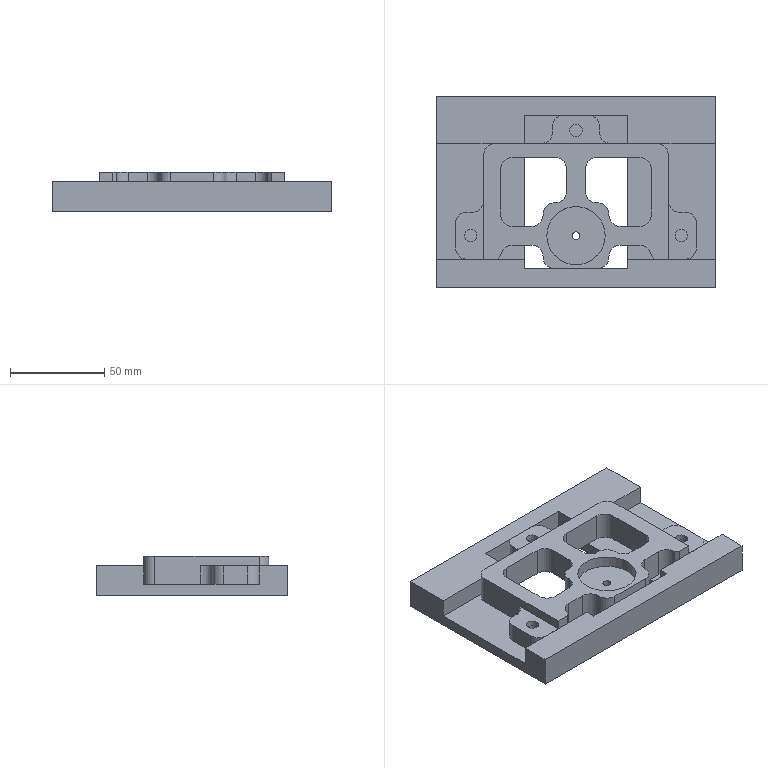NC program | NX | posted with a generic post | part box 148 x 101.5 x 21 mm
Lines 3456 to 5224 of 5700, first 1550 of 1759 lines:
(DRILLING , TOOL : D6A45)
N6898 T01 M6
N6900 G54
N6902 G17 G0 G90 X-56. Y23.25 S5000 M3
N6904 G43 Z30. H1
N6906 G94 G81 G98 Z-6. F250. R-2.
N6908 X0. Z-7. R-3.
N6910 Y-32.75 Z-6. R-2.
N6912 X56. Y23.25
N6914 G80
N6916 G0 X56. Y23.25 Z30.
N6918 M5
(DRILLING_COPY , TOOL : 4.2ZT)
N6920 T12 M6
N6922 G54
N6924 G17 G0 G90 X0. Y23.25 S2000 M3
N6926 G43 Z30. H12
N6928 G94 G83 G98 Z-16.262 F250. Q3. R-3.
N6930 G80
N6932 G0 X0. Y23.25 Z30.
N6934 M5
(DRILLING_COPY_COPY , TOOL : 6.6ZT)
N6936 T13 M6
N6938 G54
N6940 G17 G0 G90 X-56. Y23.25 S2000 M3
N6942 G43 Z30. H13
N6944 G94 G83 G98 Z-11.683 F250. Q3. R-2.
N6946 X0. Y-32.75
N6948 X56. Y23.25
N6950 G80
N6952 G0 X56. Y23.25 Z30.
N6954 M5
(ZLEVEL_PROFILE_COPY_1 , TOOL : D10)
N6956 T04 M6
N6958 G54
N6960 G17 G0 G90 X-33.9 Y-12.15 S9500 M3
N6962 G43 Z30. H4
N6964 Z-0.98
N6966 G94 G1 X-34.433 Y-12.9 F1000.
N6968 G3 X-34. Y-13.15 R0.5
N6970 G1 X-11. F2200.
N6972 G3 X-10.1 Y-12.25 R0.9
N6974 G1 Y-0.25
N6976 G3 X-10.999 Y0.65 R0.9
N6978 G1 X-11.5
N6980 G2 X-22.6 Y11.75 R11.1
N6982 G1 Y12.25
N6984 G3 X-23.5 Y13.15 R0.9
N6986 G1 X-34.
N6988 G3 X-34.9 Y12.25 R0.9
N6990 G1 Y-12.25
N6992 G3 X-34. Y-13.15 R0.9
N6994 X-33.134 Y-12.65 R1.
N6996 G1 X-32.845 Y-12.15
N6998 G0 X-33.9 Z-1.96
N7000 G1 X-34.433 Y-12.9 F1000.
N7002 G3 X-34. Y-13.15 R0.5
N7004 G1 X-11. F2200.
N7006 G3 X-10.1 Y-12.25 R0.9
N7008 G1 Y-0.25
N7010 G3 X-10.999 Y0.65 R0.9
N7012 G1 X-11.5
N7014 G2 X-22.6 Y11.75 R11.1
N7016 G1 Y12.25
N7018 G3 X-23.5 Y13.15 R0.9
N7020 G1 X-34.
N7022 G3 X-34.9 Y12.25 R0.9
N7024 G1 Y-12.25
N7026 G3 X-34. Y-13.15 R0.9
N7028 X-33.134 Y-12.65 R1.
N7030 G1 X-32.845 Y-12.15
N7032 G0 X-33.9 Z-2.94
N7034 G1 X-34.433 Y-12.9 F1000.
N7036 G3 X-34. Y-13.15 R0.5
N7038 G1 X-11. F2200.
N7040 G3 X-10.1 Y-12.25 R0.9
N7042 G1 Y-0.25
N7044 G3 X-10.999 Y0.65 R0.9
N7046 G1 X-11.5
N7048 G2 X-22.6 Y11.75 R11.1
N7050 G1 Y12.25
N7052 G3 X-23.5 Y13.15 R0.9
N7054 G1 X-34.
N7056 G3 X-34.9 Y12.25 R0.9
N7058 G1 Y-12.25
N7060 G3 X-34. Y-13.15 R0.9
N7062 X-33.134 Y-12.65 R1.
N7064 G1 X-32.845 Y-12.15
N7066 G0 X-33.9 Z-3.92
N7068 G1 X-34.433 Y-12.9 F1000.
N7070 G3 X-34. Y-13.15 R0.5
N7072 G1 X-11. F2200.
N7074 G3 X-10.1 Y-12.25 R0.9
N7076 G1 Y-0.25
N7078 G3 X-10.999 Y0.65 R0.9
N7080 G1 X-11.5
N7082 G2 X-22.6 Y11.75 R11.1
N7084 G1 Y12.25
N7086 G3 X-23.5 Y13.15 R0.9
N7088 G1 X-34.
N7090 G3 X-34.9 Y12.25 R0.9
N7092 G1 Y-12.25
N7094 G3 X-34. Y-13.15 R0.9
N7096 X-33.134 Y-12.65 R1.
N7098 G1 X-32.845 Y-12.15
N7100 G0 X-33.9 Z-4.9
N7102 G1 X-34.433 Y-12.9 F1000.
N7104 G3 X-34. Y-13.15 R0.5
N7106 G1 X-11. F2200.
N7108 G3 X-10.1 Y-12.25 R0.9
N7110 G1 Y-0.25
N7112 G3 X-10.999 Y0.65 R0.9
N7114 G1 X-11.5
N7116 G2 X-22.6 Y11.75 R11.1
N7118 G1 Y12.25
N7120 G3 X-23.5 Y13.15 R0.9
N7122 G1 X-34.
N7124 G3 X-34.9 Y12.25 R0.9
N7126 G1 Y-12.25
N7128 G3 X-34. Y-13.15 R0.9
N7130 X-33.134 Y-12.65 R1.
N7132 G1 X-32.845 Y-12.15
N7134 G0 X-33.9 Z-5.9
N7136 G1 X-34.433 Y-12.9 F1000.
N7138 G3 X-34. Y-13.15 R0.5
N7140 G1 X-11. F2200.
N7142 G3 X-10.1 Y-12.25 R0.9
N7144 G1 Y-0.25
N7146 G3 X-10.999 Y0.65 R0.9
N7148 G1 X-11.5
N7150 G2 X-22.6 Y11.75 R11.1
N7152 G1 Y12.25
N7154 G3 X-23.5 Y13.15 R0.9
N7156 G1 X-34.
N7158 G3 X-34.9 Y12.25 R0.9
N7160 G1 Y-12.25
N7162 G3 X-34. Y-13.15 R0.9
N7164 X-33.134 Y-12.65 R1.
N7166 G1 X-32.845 Y-12.15
N7168 G0 X-33.9 Z-6.844
N7170 G1 X-34.433 Y-12.9 F1000.
N7172 G3 X-34. Y-13.15 R0.5
N7174 G1 X-11. F2200.
N7176 G3 X-10.1 Y-12.25 R0.9
N7178 G1 Y-0.25
N7180 G3 X-10.999 Y0.65 R0.9
N7182 G1 X-11.5
N7184 G2 X-22.6 Y11.75 R11.1
N7186 G1 Y12.25
N7188 G3 X-23.5 Y13.15 R0.9
N7190 G1 X-34.
N7192 G3 X-34.9 Y12.25 R0.9
N7194 G1 Y-12.25
N7196 G3 X-34. Y-13.15 R0.9
N7198 X-33.134 Y-12.65 R1.
N7200 G1 X-32.845 Y-12.15
N7202 G0 X-33.9 Z-7.788
N7204 G1 X-34.433 Y-12.9 F1000.
N7206 G3 X-34. Y-13.15 R0.5
N7208 G1 X-11. F2200.
N7210 G3 X-10.1 Y-12.25 R0.9
N7212 G1 Y-0.25
N7214 G3 X-10.999 Y0.65 R0.9
N7216 G1 X-11.5
N7218 G2 X-22.6 Y11.75 R11.1
N7220 G1 Y12.25
N7222 G3 X-23.5 Y13.15 R0.9
N7224 G1 X-34.
N7226 G3 X-34.9 Y12.25 R0.9
N7228 G1 Y-12.25
N7230 G3 X-34. Y-13.15 R0.9
N7232 X-33.134 Y-12.65 R1.
N7234 G1 X-32.845 Y-12.15
N7236 G0 X-33.9 Z-8.731
N7238 G1 X-34.433 Y-12.9 F1000.
N7240 G3 X-34. Y-13.15 R0.5
N7242 G1 X-11. F2200.
N7244 G3 X-10.1 Y-12.25 R0.9
N7246 G1 Y-0.25
N7248 G3 X-10.999 Y0.65 R0.9
N7250 G1 X-11.5
N7252 G2 X-22.6 Y11.75 R11.1
N7254 G1 Y12.25
N7256 G3 X-23.5 Y13.15 R0.9
N7258 G1 X-34.
N7260 G3 X-34.9 Y12.25 R0.9
N7262 G1 Y-12.25
N7264 G3 X-34. Y-13.15 R0.9
N7266 X-33.134 Y-12.65 R1.
N7268 G1 X-32.845 Y-12.15
N7270 G0 X-33.9 Z-9.675
N7272 G1 X-34.433 Y-12.9 F1000.
N7274 G3 X-34. Y-13.15 R0.5
N7276 G1 X-11. F2200.
N7278 G3 X-10.1 Y-12.25 R0.9
N7280 G1 Y-0.25
N7282 G3 X-10.999 Y0.65 R0.9
N7284 G1 X-11.5
N7286 G2 X-22.6 Y11.75 R11.1
N7288 G1 Y12.25
N7290 G3 X-23.5 Y13.15 R0.9
N7292 G1 X-34.
N7294 G3 X-34.9 Y12.25 R0.9
N7296 G1 Y-12.25
N7298 G3 X-34. Y-13.15 R0.9
N7300 X-33.134 Y-12.65 R1.
N7302 G1 X-32.845 Y-12.15
N7304 G0 X-33.9 Z-10.619
N7306 G1 X-34.433 Y-12.9 F1000.
N7308 G3 X-34. Y-13.15 R0.5
N7310 G1 X-11. F2200.
N7312 G3 X-10.1 Y-12.25 R0.9
N7314 G1 Y-0.25
N7316 G3 X-10.999 Y0.65 R0.9
N7318 G1 X-11.5
N7320 G2 X-22.6 Y11.75 R11.1
N7322 G1 Y12.25
N7324 G3 X-23.5 Y13.15 R0.9
N7326 G1 X-34.
N7328 G3 X-34.9 Y12.25 R0.9
N7330 G1 Y-12.25
N7332 G3 X-34. Y-13.15 R0.9
N7334 X-33.134 Y-12.65 R1.
N7336 G1 X-32.845 Y-12.15
N7338 G0 X-33.9 Z-11.563
N7340 G1 X-34.433 Y-12.9 F1000.
N7342 G3 X-34. Y-13.15 R0.5
N7344 G1 X-11. F2200.
N7346 G3 X-10.1 Y-12.25 R0.9
N7348 G1 Y-0.25
N7350 G3 X-10.999 Y0.65 R0.9
N7352 G1 X-11.5
N7354 G2 X-22.6 Y11.75 R11.1
N7356 G1 Y12.25
N7358 G3 X-23.5 Y13.15 R0.9
N7360 G1 X-34.
N7362 G3 X-34.9 Y12.25 R0.9
N7364 G1 Y-12.25
N7366 G3 X-34. Y-13.15 R0.9
N7368 X-33.134 Y-12.65 R1.
N7370 G1 X-32.845 Y-12.15
N7372 G0 X-33.9 Z-12.506
N7374 G1 X-34.433 Y-12.9 F1000.
N7376 G3 X-34. Y-13.15 R0.5
N7378 G1 X-11. F2200.
N7380 G3 X-10.1 Y-12.25 R0.9
N7382 G1 Y-0.25
N7384 G3 X-10.999 Y0.65 R0.9
N7386 G1 X-11.5
N7388 G2 X-22.6 Y11.75 R11.1
N7390 G1 Y12.25
N7392 G3 X-23.5 Y13.15 R0.9
N7394 G1 X-34.
N7396 G3 X-34.9 Y12.25 R0.9
N7398 G1 Y-12.25
N7400 G3 X-34. Y-13.15 R0.9
N7402 X-33.134 Y-12.65 R1.
N7404 G1 X-32.845 Y-12.15
N7406 G0 X-33.9 Z-13.45
N7408 G1 X-34.433 Y-12.9 F1000.
N7410 G3 X-34. Y-13.15 R0.5
N7412 G1 X-11. F2200.
N7414 G3 X-10.1 Y-12.25 R0.9
N7416 G1 Y-0.25
N7418 G3 X-10.999 Y0.65 R0.9
N7420 G1 X-11.5
N7422 G2 X-22.6 Y11.75 R11.1
N7424 G1 Y12.25
N7426 G3 X-23.5 Y13.15 R0.9
N7428 G1 X-34.
N7430 G3 X-34.9 Y12.25 R0.9
N7432 G1 Y-12.25
N7434 G3 X-34. Y-13.15 R0.9
N7436 X-33.134 Y-12.65 R1.
N7438 G1 X-32.845 Y-12.15
N7440 G0 X-33.9 Z-14.394
N7442 G1 X-34.433 Y-12.9 F1000.
N7444 G3 X-34. Y-13.15 R0.5
N7446 G1 X-11. F2200.
N7448 G3 X-10.1 Y-12.25 R0.9
N7450 G1 Y-0.25
N7452 G3 X-10.999 Y0.65 R0.9
N7454 G1 X-11.5
N7456 G2 X-22.6 Y11.75 R11.1
N7458 G1 Y12.25
N7460 G3 X-23.5 Y13.15 R0.9
N7462 G1 X-34.
N7464 G3 X-34.9 Y12.25 R0.9
N7466 G1 Y-12.25
N7468 G3 X-34. Y-13.15 R0.9
N7470 X-33.134 Y-12.65 R1.
N7472 G1 X-32.845 Y-12.15
N7474 G0 X-33.9 Z-15.338
N7476 G1 X-34.433 Y-12.9 F1000.
N7478 G3 X-34. Y-13.15 R0.5
N7480 G1 X-11. F2200.
N7482 G3 X-10.1 Y-12.25 R0.9
N7484 G1 Y-0.25
N7486 G3 X-10.999 Y0.65 R0.9
N7488 G1 X-11.5
N7490 G2 X-22.6 Y11.75 R11.1
N7492 G1 Y12.25
N7494 G3 X-23.5 Y13.15 R0.9
N7496 G1 X-34.
N7498 G3 X-34.9 Y12.25 R0.9
N7500 G1 Y-12.25
N7502 G3 X-34. Y-13.15 R0.9
N7504 X-33.134 Y-12.65 R1.
N7506 G1 X-32.845 Y-12.15
N7508 G0 X-33.9 Z-16.281
N7510 G1 X-34.433 Y-12.9 F1000.
N7512 G3 X-34. Y-13.15 R0.5
N7514 G1 X-11. F2200.
N7516 G3 X-10.1 Y-12.25 R0.9
N7518 G1 Y-0.25
N7520 G3 X-10.999 Y0.65 R0.9
N7522 G1 X-11.5
N7524 G2 X-22.6 Y11.75 R11.1
N7526 G1 Y12.25
N7528 G3 X-23.5 Y13.15 R0.9
N7530 G1 X-34.
N7532 G3 X-34.9 Y12.25 R0.9
N7534 G1 Y-12.25
N7536 G3 X-34. Y-13.15 R0.9
N7538 X-33.134 Y-12.65 R1.
N7540 G1 X-32.845 Y-12.15
N7542 G0 X-33.9 Z-17.225
N7544 G1 X-34.433 Y-12.9 F1000.
N7546 G3 X-34. Y-13.15 R0.5
N7548 G1 X-11. F2200.
N7550 G3 X-10.1 Y-12.25 R0.9
N7552 G1 Y-0.25
N7554 G3 X-10.999 Y0.65 R0.9
N7556 G1 X-11.5
N7558 G2 X-22.6 Y11.75 R11.1
N7560 G1 Y12.25
N7562 G3 X-23.5 Y13.15 R0.9
N7564 G1 X-34.
N7566 G3 X-34.9 Y12.25 R0.9
N7568 G1 Y-12.25
N7570 G3 X-34. Y-13.15 R0.9
N7572 X-33.134 Y-12.65 R1.
N7574 G1 X-32.845 Y-12.15
N7576 G0 X-33.9 Z-18.169
N7578 G1 X-34.433 Y-12.9 F1000.
N7580 G3 X-34. Y-13.15 R0.5
N7582 G1 X-11. F2200.
N7584 G3 X-10.1 Y-12.25 R0.9
N7586 G1 Y-0.25
N7588 G3 X-10.999 Y0.65 R0.9
N7590 G1 X-11.5
N7592 G2 X-22.6 Y11.75 R11.1
N7594 G1 Y12.25
N7596 G3 X-23.5 Y13.15 R0.9
N7598 G1 X-34.
N7600 G3 X-34.9 Y12.25 R0.9
N7602 G1 Y-12.25
N7604 G3 X-34. Y-13.15 R0.9
N7606 X-33.134 Y-12.65 R1.
N7608 G1 X-32.845 Y-12.15
N7610 G0 X-33.9 Z-19.113
N7612 G1 X-34.433 Y-12.9 F1000.
N7614 G3 X-34. Y-13.15 R0.5
N7616 G1 X-11. F2200.
N7618 G3 X-10.1 Y-12.25 R0.9
N7620 G1 Y-0.25
N7622 G3 X-10.999 Y0.65 R0.9
N7624 G1 X-11.5
N7626 G2 X-22.6 Y11.75 R11.1
N7628 G1 Y12.25
N7630 G3 X-23.5 Y13.15 R0.9
N7632 G1 X-34.
N7634 G3 X-34.9 Y12.25 R0.9
N7636 G1 Y-12.25
N7638 G3 X-34. Y-13.15 R0.9
N7640 X-33.134 Y-12.65 R1.
N7642 G1 X-32.845 Y-12.15
N7644 G0 X-33.9 Z-20.056
N7646 G1 X-34.433 Y-12.9 F1000.
N7648 G3 X-34. Y-13.15 R0.5
N7650 G1 X-11. F2200.
N7652 G3 X-10.1 Y-12.25 R0.9
N7654 G1 Y-0.25
N7656 G3 X-10.999 Y0.65 R0.9
N7658 G1 X-11.5
N7660 G2 X-22.6 Y11.75 R11.1
N7662 G1 Y12.25
N7664 G3 X-23.5 Y13.15 R0.9
N7666 G1 X-34.
N7668 G3 X-34.9 Y12.25 R0.9
N7670 G1 Y-12.25
N7672 G3 X-34. Y-13.15 R0.9
N7674 X-33.134 Y-12.65 R1.
N7676 G1 X-32.845 Y-12.15
N7678 G0 X-33.9 Z-21.
N7680 G1 X-34.433 Y-12.9 F1000.
N7682 G3 X-34. Y-13.15 R0.5
N7684 G1 X-11. F2200.
N7686 G3 X-10.1 Y-12.25 R0.9
N7688 G1 Y-0.25
N7690 G3 X-10.999 Y0.65 R0.9
N7692 G1 X-11.5
N7694 G2 X-22.6 Y11.75 R11.1
N7696 G1 Y12.25
N7698 G3 X-23.5 Y13.15 R0.9
N7700 G1 X-34.
N7702 G3 X-34.9 Y12.25 R0.9
N7704 G1 Y-12.25
N7706 G3 X-34. Y-13.15 R0.9
N7708 X-33.134 Y-12.65 R1.
N7710 G1 X-32.845 Y-12.15
N7712 G0 Z30.
N7714 X11.1
N7716 Z-0.98
N7718 G1 X10.567 Y-12.9 F1000.
N7720 G3 X11. Y-13.15 R0.5
N7722 G1 X34. F2200.
N7724 G3 X34.9 Y-12.25 R0.9
N7726 G1 Y12.25
N7728 G3 X34. Y13.15 R0.9
N7730 G1 X23.5
N7732 G3 X22.6 Y12.25 R0.9
N7734 G1 Y11.75
N7736 G2 X11.5 Y0.65 R11.1
N7738 G1 X11.
N7740 G3 X10.1 Y-0.25 R0.9
N7742 G1 Y-12.25
N7744 G3 X11. Y-13.15 R0.9
N7746 X11.866 Y-12.65 R1.
N7748 G1 X12.155 Y-12.15
N7750 G0 X11.1 Z-1.96
N7752 G1 X10.567 Y-12.9 F1000.
N7754 G3 X11. Y-13.15 R0.5
N7756 G1 X34. F2200.
N7758 G3 X34.9 Y-12.25 R0.9
N7760 G1 Y12.25
N7762 G3 X34. Y13.15 R0.9
N7764 G1 X23.5
N7766 G3 X22.6 Y12.25 R0.9
N7768 G1 Y11.75
N7770 G2 X11.5 Y0.65 R11.1
N7772 G1 X11.
N7774 G3 X10.1 Y-0.25 R0.9
N7776 G1 Y-12.25
N7778 G3 X11. Y-13.15 R0.9
N7780 X11.866 Y-12.65 R1.
N7782 G1 X12.155 Y-12.15
N7784 G0 X11.1 Z-2.94
N7786 G1 X10.567 Y-12.9 F1000.
N7788 G3 X11. Y-13.15 R0.5
N7790 G1 X34. F2200.
N7792 G3 X34.9 Y-12.25 R0.9
N7794 G1 Y12.25
N7796 G3 X34. Y13.15 R0.9
N7798 G1 X23.5
N7800 G3 X22.6 Y12.25 R0.9
N7802 G1 Y11.75
N7804 G2 X11.5 Y0.65 R11.1
N7806 G1 X11.
N7808 G3 X10.1 Y-0.25 R0.9
N7810 G1 Y-12.25
N7812 G3 X11. Y-13.15 R0.9
N7814 X11.866 Y-12.65 R1.
N7816 G1 X12.155 Y-12.15
N7818 G0 X11.1 Z-3.92
N7820 G1 X10.567 Y-12.9 F1000.
N7822 G3 X11. Y-13.15 R0.5
N7824 G1 X34. F2200.
N7826 G3 X34.9 Y-12.25 R0.9
N7828 G1 Y12.25
N7830 G3 X34. Y13.15 R0.9
N7832 G1 X23.5
N7834 G3 X22.6 Y12.25 R0.9
N7836 G1 Y11.75
N7838 G2 X11.5 Y0.65 R11.1
N7840 G1 X11.
N7842 G3 X10.1 Y-0.25 R0.9
N7844 G1 Y-12.25
N7846 G3 X11. Y-13.15 R0.9
N7848 X11.866 Y-12.65 R1.
N7850 G1 X12.155 Y-12.15
N7852 G0 X11.1 Z-4.9
N7854 G1 X10.567 Y-12.9 F1000.
N7856 G3 X11. Y-13.15 R0.5
N7858 G1 X34. F2200.
N7860 G3 X34.9 Y-12.25 R0.9
N7862 G1 Y12.25
N7864 G3 X34. Y13.15 R0.9
N7866 G1 X23.5
N7868 G3 X22.6 Y12.25 R0.9
N7870 G1 Y11.75
N7872 G2 X11.5 Y0.65 R11.1
N7874 G1 X11.
N7876 G3 X10.1 Y-0.25 R0.9
N7878 G1 Y-12.25
N7880 G3 X11. Y-13.15 R0.9
N7882 X11.866 Y-12.65 R1.
N7884 G1 X12.155 Y-12.15
N7886 G0 X11.1 Z-5.9
N7888 G1 X10.567 Y-12.9 F1000.
N7890 G3 X11. Y-13.15 R0.5
N7892 G1 X34. F2200.
N7894 G3 X34.9 Y-12.25 R0.9
N7896 G1 Y12.25
N7898 G3 X34. Y13.15 R0.9
N7900 G1 X23.5
N7902 G3 X22.6 Y12.25 R0.9
N7904 G1 Y11.75
N7906 G2 X11.5 Y0.65 R11.1
N7908 G1 X11.
N7910 G3 X10.1 Y-0.25 R0.9
N7912 G1 Y-12.25
N7914 G3 X11. Y-13.15 R0.9
N7916 X11.866 Y-12.65 R1.
N7918 G1 X12.155 Y-12.15
N7920 G0 X11.1 Z-6.844
N7922 G1 X10.567 Y-12.9 F1000.
N7924 G3 X11. Y-13.15 R0.5
N7926 G1 X34. F2200.
N7928 G3 X34.9 Y-12.25 R0.9
N7930 G1 Y12.25
N7932 G3 X34. Y13.15 R0.9
N7934 G1 X23.5
N7936 G3 X22.6 Y12.25 R0.9
N7938 G1 Y11.75
N7940 G2 X11.5 Y0.65 R11.1
N7942 G1 X11.
N7944 G3 X10.1 Y-0.25 R0.9
N7946 G1 Y-12.25
N7948 G3 X11. Y-13.15 R0.9
N7950 X11.866 Y-12.65 R1.
N7952 G1 X12.155 Y-12.15
N7954 G0 X11.1 Z-7.788
N7956 G1 X10.567 Y-12.9 F1000.
N7958 G3 X11. Y-13.15 R0.5
N7960 G1 X34. F2200.
N7962 G3 X34.9 Y-12.25 R0.9
N7964 G1 Y12.25
N7966 G3 X34. Y13.15 R0.9
N7968 G1 X23.5
N7970 G3 X22.6 Y12.25 R0.9
N7972 G1 Y11.75
N7974 G2 X11.5 Y0.65 R11.1
N7976 G1 X11.
N7978 G3 X10.1 Y-0.25 R0.9
N7980 G1 Y-12.25
N7982 G3 X11. Y-13.15 R0.9
N7984 X11.866 Y-12.65 R1.
N7986 G1 X12.155 Y-12.15
N7988 G0 X11.1 Z-8.731
N7990 G1 X10.567 Y-12.9 F1000.
N7992 G3 X11. Y-13.15 R0.5
N7994 G1 X34. F2200.
N7996 G3 X34.9 Y-12.25 R0.9
N7998 G1 Y12.25
N8000 G3 X34. Y13.15 R0.9
N8002 G1 X23.5
N8004 G3 X22.6 Y12.25 R0.9
N8006 G1 Y11.75
N8008 G2 X11.5 Y0.65 R11.1
N8010 G1 X11.
N8012 G3 X10.1 Y-0.25 R0.9
N8014 G1 Y-12.25
N8016 G3 X11. Y-13.15 R0.9
N8018 X11.866 Y-12.65 R1.
N8020 G1 X12.155 Y-12.15
N8022 G0 X11.1 Z-9.675
N8024 G1 X10.567 Y-12.9 F1000.
N8026 G3 X11. Y-13.15 R0.5
N8028 G1 X34. F2200.
N8030 G3 X34.9 Y-12.25 R0.9
N8032 G1 Y12.25
N8034 G3 X34. Y13.15 R0.9
N8036 G1 X23.5
N8038 G3 X22.6 Y12.25 R0.9
N8040 G1 Y11.75
N8042 G2 X11.5 Y0.65 R11.1
N8044 G1 X11.
N8046 G3 X10.1 Y-0.25 R0.9
N8048 G1 Y-12.25
N8050 G3 X11. Y-13.15 R0.9
N8052 X11.866 Y-12.65 R1.
N8054 G1 X12.155 Y-12.15
N8056 G0 X11.1 Z-10.619
N8058 G1 X10.567 Y-12.9 F1000.
N8060 G3 X11. Y-13.15 R0.5
N8062 G1 X34. F2200.
N8064 G3 X34.9 Y-12.25 R0.9
N8066 G1 Y12.25
N8068 G3 X34. Y13.15 R0.9
N8070 G1 X23.5
N8072 G3 X22.6 Y12.25 R0.9
N8074 G1 Y11.75
N8076 G2 X11.5 Y0.65 R11.1
N8078 G1 X11.
N8080 G3 X10.1 Y-0.25 R0.9
N8082 G1 Y-12.25
N8084 G3 X11. Y-13.15 R0.9
N8086 X11.866 Y-12.65 R1.
N8088 G1 X12.155 Y-12.15
N8090 G0 X11.1 Z-11.563
N8092 G1 X10.567 Y-12.9 F1000.
N8094 G3 X11. Y-13.15 R0.5
N8096 G1 X34. F2200.
N8098 G3 X34.9 Y-12.25 R0.9
N8100 G1 Y12.25
N8102 G3 X34. Y13.15 R0.9
N8104 G1 X23.5
N8106 G3 X22.6 Y12.25 R0.9
N8108 G1 Y11.75
N8110 G2 X11.5 Y0.65 R11.1
N8112 G1 X11.
N8114 G3 X10.1 Y-0.25 R0.9
N8116 G1 Y-12.25
N8118 G3 X11. Y-13.15 R0.9
N8120 X11.866 Y-12.65 R1.
N8122 G1 X12.155 Y-12.15
N8124 G0 X11.1 Z-12.506
N8126 G1 X10.567 Y-12.9 F1000.
N8128 G3 X11. Y-13.15 R0.5
N8130 G1 X34. F2200.
N8132 G3 X34.9 Y-12.25 R0.9
N8134 G1 Y12.25
N8136 G3 X34. Y13.15 R0.9
N8138 G1 X23.5
N8140 G3 X22.6 Y12.25 R0.9
N8142 G1 Y11.75
N8144 G2 X11.5 Y0.65 R11.1
N8146 G1 X11.
N8148 G3 X10.1 Y-0.25 R0.9
N8150 G1 Y-12.25
N8152 G3 X11. Y-13.15 R0.9
N8154 X11.866 Y-12.65 R1.
N8156 G1 X12.155 Y-12.15
N8158 G0 X11.1 Z-13.45
N8160 G1 X10.567 Y-12.9 F1000.
N8162 G3 X11. Y-13.15 R0.5
N8164 G1 X34. F2200.
N8166 G3 X34.9 Y-12.25 R0.9
N8168 G1 Y12.25
N8170 G3 X34. Y13.15 R0.9
N8172 G1 X23.5
N8174 G3 X22.6 Y12.25 R0.9
N8176 G1 Y11.75
N8178 G2 X11.5 Y0.65 R11.1
N8180 G1 X11.
N8182 G3 X10.1 Y-0.25 R0.9
N8184 G1 Y-12.25
N8186 G3 X11. Y-13.15 R0.9
N8188 X11.866 Y-12.65 R1.
N8190 G1 X12.155 Y-12.15
N8192 G0 X11.1 Z-14.394
N8194 G1 X10.567 Y-12.9 F1000.
N8196 G3 X11. Y-13.15 R0.5
N8198 G1 X34. F2200.
N8200 G3 X34.9 Y-12.25 R0.9
N8202 G1 Y12.25
N8204 G3 X34. Y13.15 R0.9
N8206 G1 X23.5
N8208 G3 X22.6 Y12.25 R0.9
N8210 G1 Y11.75
N8212 G2 X11.5 Y0.65 R11.1
N8214 G1 X11.
N8216 G3 X10.1 Y-0.25 R0.9
N8218 G1 Y-12.25
N8220 G3 X11. Y-13.15 R0.9
N8222 X11.866 Y-12.65 R1.
N8224 G1 X12.155 Y-12.15
N8226 G0 X11.1 Z-15.338
N8228 G1 X10.567 Y-12.9 F1000.
N8230 G3 X11. Y-13.15 R0.5
N8232 G1 X34. F2200.
N8234 G3 X34.9 Y-12.25 R0.9
N8236 G1 Y12.25
N8238 G3 X34. Y13.15 R0.9
N8240 G1 X23.5
N8242 G3 X22.6 Y12.25 R0.9
N8244 G1 Y11.75
N8246 G2 X11.5 Y0.65 R11.1
N8248 G1 X11.
N8250 G3 X10.1 Y-0.25 R0.9
N8252 G1 Y-12.25
N8254 G3 X11. Y-13.15 R0.9
N8256 X11.866 Y-12.65 R1.
N8258 G1 X12.155 Y-12.15
N8260 G0 X11.1 Z-16.281
N8262 G1 X10.567 Y-12.9 F1000.
N8264 G3 X11. Y-13.15 R0.5
N8266 G1 X34. F2200.
N8268 G3 X34.9 Y-12.25 R0.9
N8270 G1 Y12.25
N8272 G3 X34. Y13.15 R0.9
N8274 G1 X23.5
N8276 G3 X22.6 Y12.25 R0.9
N8278 G1 Y11.75
N8280 G2 X11.5 Y0.65 R11.1
N8282 G1 X11.
N8284 G3 X10.1 Y-0.25 R0.9
N8286 G1 Y-12.25
N8288 G3 X11. Y-13.15 R0.9
N8290 X11.866 Y-12.65 R1.
N8292 G1 X12.155 Y-12.15
N8294 G0 X11.1 Z-17.225
N8296 G1 X10.567 Y-12.9 F1000.
N8298 G3 X11. Y-13.15 R0.5
N8300 G1 X34. F2200.
N8302 G3 X34.9 Y-12.25 R0.9
N8304 G1 Y12.25
N8306 G3 X34. Y13.15 R0.9
N8308 G1 X23.5
N8310 G3 X22.6 Y12.25 R0.9
N8312 G1 Y11.75
N8314 G2 X11.5 Y0.65 R11.1
N8316 G1 X11.
N8318 G3 X10.1 Y-0.25 R0.9
N8320 G1 Y-12.25
N8322 G3 X11. Y-13.15 R0.9
N8324 X11.866 Y-12.65 R1.
N8326 G1 X12.155 Y-12.15
N8328 G0 X11.1 Z-18.169
N8330 G1 X10.567 Y-12.9 F1000.
N8332 G3 X11. Y-13.15 R0.5
N8334 G1 X34. F2200.
N8336 G3 X34.9 Y-12.25 R0.9
N8338 G1 Y12.25
N8340 G3 X34. Y13.15 R0.9
N8342 G1 X23.5
N8344 G3 X22.6 Y12.25 R0.9
N8346 G1 Y11.75
N8348 G2 X11.5 Y0.65 R11.1
N8350 G1 X11.
N8352 G3 X10.1 Y-0.25 R0.9
N8354 G1 Y-12.25
N8356 G3 X11. Y-13.15 R0.9
N8358 X11.866 Y-12.65 R1.
N8360 G1 X12.155 Y-12.15
N8362 G0 X11.1 Z-19.113
N8364 G1 X10.567 Y-12.9 F1000.
N8366 G3 X11. Y-13.15 R0.5
N8368 G1 X34. F2200.
N8370 G3 X34.9 Y-12.25 R0.9
N8372 G1 Y12.25
N8374 G3 X34. Y13.15 R0.9
N8376 G1 X23.5
N8378 G3 X22.6 Y12.25 R0.9
N8380 G1 Y11.75
N8382 G2 X11.5 Y0.65 R11.1
N8384 G1 X11.
N8386 G3 X10.1 Y-0.25 R0.9
N8388 G1 Y-12.25
N8390 G3 X11. Y-13.15 R0.9
N8392 X11.866 Y-12.65 R1.
N8394 G1 X12.155 Y-12.15
N8396 G0 X11.1 Z-20.056
N8398 G1 X10.567 Y-12.9 F1000.
N8400 G3 X11. Y-13.15 R0.5
N8402 G1 X34. F2200.
N8404 G3 X34.9 Y-12.25 R0.9
N8406 G1 Y12.25
N8408 G3 X34. Y13.15 R0.9
N8410 G1 X23.5
N8412 G3 X22.6 Y12.25 R0.9
N8414 G1 Y11.75
N8416 G2 X11.5 Y0.65 R11.1
N8418 G1 X11.
N8420 G3 X10.1 Y-0.25 R0.9
N8422 G1 Y-12.25
N8424 G3 X11. Y-13.15 R0.9
N8426 X11.866 Y-12.65 R1.
N8428 G1 X12.155 Y-12.15
N8430 G0 X11.1 Z-21.
N8432 G1 X10.567 Y-12.9 F1000.
N8434 G3 X11. Y-13.15 R0.5
N8436 G1 X34. F2200.
N8438 G3 X34.9 Y-12.25 R0.9
N8440 G1 Y12.25
N8442 G3 X34. Y13.15 R0.9
N8444 G1 X23.5
N8446 G3 X22.6 Y12.25 R0.9
N8448 G1 Y11.75
N8450 G2 X11.5 Y0.65 R11.1
N8452 G1 X11.
N8454 G3 X10.1 Y-0.25 R0.9
N8456 G1 Y-12.25
N8458 G3 X11. Y-13.15 R0.9
N8460 X11.866 Y-12.65 R1.
N8462 G1 X12.155 Y-12.15
N8464 G0 Z30.
N8466 X1.199 Y32.573
N8468 Z-0.98
N8470 G1 X0.866 Y33.15 F1000.
N8472 G3 X0. Y33.65 R1.
N8474 X-10.4 Y23.25 R10.4 F2200.
N8476 X0. Y33.65 R-10.4
N8478 X-0.866 Y33.15 R1.
N8480 G1 X-1.199 Y32.573
N8482 G0 X1.199 Z-1.96
N8484 G1 X0.866 Y33.15 F1000.
N8486 G3 X0. Y33.65 R1.
N8488 X-10.4 Y23.25 R10.4 F2200.
N8490 X0. Y33.65 R-10.4
N8492 X-0.866 Y33.15 R1.
N8494 G1 X-1.199 Y32.573
N8496 G0 X1.199 Z-2.94
N8498 G1 X0.866 Y33.15 F1000.
N8500 G3 X0. Y33.65 R1.
N8502 X-10.4 Y23.25 R10.4 F2200.
N8504 X0. Y33.65 R-10.4
N8506 X-0.866 Y33.15 R1.
N8508 G1 X-1.199 Y32.573
N8510 G0 X1.199 Z-3.92
N8512 G1 X0.866 Y33.15 F1000.
N8514 G3 X0. Y33.65 R1.
N8516 X-10.4 Y23.25 R10.4 F2200.
N8518 X0. Y33.65 R-10.4
N8520 X-0.866 Y33.15 R1.
N8522 G1 X-1.199 Y32.573
N8524 G0 X1.199 Z-4.9
N8526 G1 X0.866 Y33.15 F1000.
N8528 G3 X0. Y33.65 R1.
N8530 X-10.4 Y23.25 R10.4 F2200.
N8532 X0. Y33.65 R-10.4
N8534 X-0.866 Y33.15 R1.
N8536 G1 X-1.199 Y32.573
N8538 G0 X1.199 Z-5.9
N8540 G1 X0.866 Y33.15 F1000.
N8542 G3 X0. Y33.65 R1.
N8544 X-10.4 Y23.25 R10.4 F2200.
N8546 X0. Y33.65 R-10.4
N8548 X-0.866 Y33.15 R1.
N8550 G1 X-1.199 Y32.573
N8552 G0 Z30.
(ZLEVEL_PROFILE , TOOL : D10)
N8554 X44.124 Y-31.798
N8556 Z-1.
N8558 G1 X43.866 Y-31.35 F1000.
N8560 G3 X43. Y-30.85 R1.
N8562 G1 X-43. F2200.
N8564 G2 X-54.1 Y-19.75 R11.1
N8566 G1 Y35.75
N8568 G2 X-49. Y40.85 R5.1
N8570 G1 X-41.984
N8572 G2 X-38.493 Y39.467 R5.1
N8574 G1 X-36.497 Y37.592
N8576 G2 X-34.898 Y34.194 R5.1
N8578 G3 X-34. Y33.35 R0.9
N8580 G1 X-23.5
N8582 G3 X-22.6 Y34.25 R0.9
N8584 G1 Y34.75
N8586 G2 X-11.5 Y45.85 R11.1
N8588 G1 X11.5
N8590 G2 X22.6 Y34.75 R11.1
N8592 G1 Y34.25
N8594 G3 X23.5 Y33.35 R0.9
N8596 G1 X34.
N8598 G3 X34.898 Y34.194 R0.9
N8600 G2 X36.497 Y37.592 R5.1
N8602 G1 X38.493 Y39.467
N8604 G2 X41.984 Y40.85 R5.1
N8606 G1 X49.
N8608 G2 X54.1 Y35.75 R5.1
N8610 G1 Y-19.75
N8612 G2 X43. Y-30.85 R11.1
N8614 G3 X42.134 Y-31.35 R1.
N8616 G1 X41.845 Y-31.85
N8618 G0 X44.124 Y-31.798 Z-2.
N8620 G1 X43.866 Y-31.35 F1000.
N8622 G3 X43. Y-30.85 R1.
N8624 G1 X-43. F2200.
N8626 G2 X-54.1 Y-19.75 R11.1
N8628 G1 Y35.75
N8630 G2 X-49. Y40.85 R5.1
N8632 G1 X-41.984
N8634 G2 X-38.493 Y39.467 R5.1
N8636 G1 X-36.497 Y37.592
N8638 G2 X-34.898 Y34.194 R5.1
N8640 G3 X-34. Y33.35 R0.9
N8642 G1 X-23.5
N8644 G3 X-22.6 Y34.25 R0.9
N8646 G1 Y34.75
N8648 G2 X-11.5 Y45.85 R11.1
N8650 G1 X11.5
N8652 G2 X22.6 Y34.75 R11.1
N8654 G1 Y34.25
N8656 G3 X23.5 Y33.35 R0.9
N8658 G1 X34.
N8660 G3 X34.898 Y34.194 R0.9
N8662 G2 X36.497 Y37.592 R5.1
N8664 G1 X38.493 Y39.467
N8666 G2 X41.984 Y40.85 R5.1
N8668 G1 X49.
N8670 G2 X54.1 Y35.75 R5.1
N8672 G1 Y-19.75
N8674 G2 X43. Y-30.85 R11.1
N8676 G3 X42.134 Y-31.35 R1.
N8678 G1 X41.845 Y-31.85
N8680 G0 X44.124 Y-31.798 Z-3.
N8682 G1 X43.866 Y-31.35 F1000.
N8684 G3 X43. Y-30.85 R1.
N8686 G1 X-43. F2200.
N8688 G2 X-54.1 Y-19.75 R11.1
N8690 G1 Y35.75
N8692 G2 X-49. Y40.85 R5.1
N8694 G1 X-41.984
N8696 G2 X-38.493 Y39.467 R5.1
N8698 G1 X-36.497 Y37.592
N8700 G2 X-34.898 Y34.194 R5.1
N8702 G3 X-34. Y33.35 R0.9
N8704 G1 X-23.5
N8706 G3 X-22.6 Y34.25 R0.9
N8708 G1 Y34.75
N8710 G2 X-11.5 Y45.85 R11.1
N8712 G1 X11.5
N8714 G2 X22.6 Y34.75 R11.1
N8716 G1 Y34.25
N8718 G3 X23.5 Y33.35 R0.9
N8720 G1 X34.
N8722 G3 X34.898 Y34.194 R0.9
N8724 G2 X36.497 Y37.592 R5.1
N8726 G1 X38.493 Y39.467
N8728 G2 X41.984 Y40.85 R5.1
N8730 G1 X49.
N8732 G2 X54.1 Y35.75 R5.1
N8734 G1 Y-19.75
N8736 G2 X43. Y-30.85 R11.1
N8738 G3 X42.134 Y-31.35 R1.
N8740 G1 X41.845 Y-31.85
N8742 G0 X44.124 Y-31.798 Z-4.
N8744 G1 X43.866 Y-31.35 F1000.
N8746 G3 X43. Y-30.85 R1.
N8748 G1 X-43. F2200.
N8750 G2 X-54.1 Y-19.75 R11.1
N8752 G1 Y35.75
N8754 G2 X-49. Y40.85 R5.1
N8756 G1 X-41.984
N8758 G2 X-38.493 Y39.467 R5.1
N8760 G1 X-36.497 Y37.592
N8762 G2 X-34.898 Y34.194 R5.1
N8764 G3 X-34. Y33.35 R0.9
N8766 G1 X-23.5
N8768 G3 X-22.6 Y34.25 R0.9
N8770 G1 Y34.75
N8772 G2 X-11.5 Y45.85 R11.1
N8774 G1 X11.5
N8776 G2 X22.6 Y34.75 R11.1
N8778 G1 Y34.25
N8780 G3 X23.5 Y33.35 R0.9
N8782 G1 X34.
N8784 G3 X34.898 Y34.194 R0.9
N8786 G2 X36.497 Y37.592 R5.1
N8788 G1 X38.493 Y39.467
N8790 G2 X41.984 Y40.85 R5.1
N8792 G1 X49.
N8794 G2 X54.1 Y35.75 R5.1
N8796 G1 Y-19.75
N8798 G2 X43. Y-30.85 R11.1
N8800 G3 X42.134 Y-31.35 R1.
N8802 G1 X41.845 Y-31.85
N8804 G0 X44.124 Y-31.798 Z-5.
N8806 G1 X43.866 Y-31.35 F1000.
N8808 G3 X43. Y-30.85 R1.
N8810 G1 X18.5 F2200.
N8812 G3 X17.6 Y-31.75 R0.9
N8814 G1 Y-34.75
N8816 G2 X6.5 Y-45.85 R11.1
N8818 G1 X-6.5
N8820 G2 X-17.6 Y-34.75 R11.1
N8822 G1 Y-31.75
N8824 G3 X-18.5 Y-30.85 R0.9
N8826 G1 X-43.
N8828 G2 X-54.1 Y-19.75 R11.1
N8830 G1 Y4.75
N8832 G3 X-55. Y5.65 R0.9
N8834 G1 X-58.
N8836 G2 X-69.1 Y16.75 R11.1
N8838 G1 Y29.75
N8840 G2 X-58. Y40.85 R11.1
N8842 G1 X-41.984
N8844 G2 X-38.493 Y39.467 R5.1
N8846 G1 X-36.497 Y37.592
N8848 G2 X-34.898 Y34.194 R5.1
N8850 G3 X-34. Y33.35 R0.9
N8852 G1 X-23.5
N8854 G3 X-22.6 Y34.25 R0.9
N8856 G1 Y34.75
N8858 G2 X-11.5 Y45.85 R11.1
N8860 G1 X11.5
N8862 G2 X22.6 Y34.75 R11.1
N8864 G1 Y34.25
N8866 G3 X23.5 Y33.35 R0.9
N8868 G1 X34.
N8870 G3 X34.898 Y34.194 R0.9
N8872 G2 X36.497 Y37.592 R5.1
N8874 G1 X38.493 Y39.467
N8876 G2 X41.984 Y40.85 R5.1
N8878 G1 X58.
N8880 G2 X69.1 Y29.75 R11.1
N8882 G1 Y16.75
N8884 G2 X58. Y5.65 R11.1
N8886 G1 X55.
N8888 G3 X54.1 Y4.75 R0.9
N8890 G1 Y-19.75
N8892 G2 X43. Y-30.85 R11.1
N8894 G3 X42.134 Y-31.35 R1.
N8896 G1 X41.845 Y-31.85
N8898 G0 X44.124 Y-31.798 Z-6.
N8900 G1 X43.866 Y-31.35 F1000.
N8902 G3 X43. Y-30.85 R1.
N8904 G1 X18.5 F2200.
N8906 G3 X17.6 Y-31.75 R0.9
N8908 G1 Y-34.75
N8910 G2 X6.5 Y-45.85 R11.1
N8912 G1 X-6.5
N8914 G2 X-17.6 Y-34.75 R11.1
N8916 G1 Y-31.75
N8918 G3 X-18.5 Y-30.85 R0.9
N8920 G1 X-43.
N8922 G2 X-54.1 Y-19.75 R11.1
N8924 G1 Y4.75
N8926 G3 X-55. Y5.65 R0.9
N8928 G1 X-58.
N8930 G2 X-69.1 Y16.75 R11.1
N8932 G1 Y29.75
N8934 G2 X-58. Y40.85 R11.1
N8936 G1 X-41.984
N8938 G2 X-38.493 Y39.467 R5.1
N8940 G1 X-36.497 Y37.592
N8942 G2 X-34.898 Y34.194 R5.1
N8944 G3 X-34. Y33.35 R0.9
N8946 G1 X-23.5
N8948 G3 X-22.6 Y34.25 R0.9
N8950 G1 Y34.75
N8952 G2 X-11.5 Y45.85 R11.1
N8954 G1 X11.5
N8956 G2 X22.6 Y34.75 R11.1
N8958 G1 Y34.25
N8960 G3 X23.5 Y33.35 R0.9
N8962 G1 X34.
N8964 G3 X34.898 Y34.194 R0.9
N8966 G2 X36.497 Y37.592 R5.1
N8968 G1 X38.493 Y39.467
N8970 G2 X41.984 Y40.85 R5.1
N8972 G1 X58.
N8974 G2 X69.1 Y29.75 R11.1
N8976 G1 Y16.75
N8978 G2 X58. Y5.65 R11.1
N8980 G1 X55.
N8982 G3 X54.1 Y4.75 R0.9
N8984 G1 Y-19.75
N8986 G2 X43. Y-30.85 R11.1
N8988 G3 X42.134 Y-31.35 R1.
N8990 G1 X41.845 Y-31.85
N8992 G0 X44.124 Y-31.798 Z-7.
N8994 G1 X43.866 Y-31.35 F1000.
N8996 G3 X43. Y-30.85 R1.
N8998 G1 X18.5 F2200.
N9000 G3 X17.6 Y-31.75 R0.9
N9002 G1 Y-34.75
N9004 G2 X6.5 Y-45.85 R11.1
N9006 G1 X-6.5
N9008 G2 X-17.6 Y-34.75 R11.1
N9010 G1 Y-31.75
N9012 G3 X-18.5 Y-30.85 R0.9
N9014 G1 X-43.
N9016 G2 X-54.1 Y-19.75 R11.1
N9018 G1 Y4.75
N9020 G3 X-55. Y5.65 R0.9
N9022 G1 X-58.
N9024 G2 X-69.1 Y16.75 R11.1
N9026 G1 Y29.75
N9028 G2 X-58. Y40.85 R11.1
N9030 G1 X-41.984
N9032 G2 X-38.493 Y39.467 R5.1
N9034 G1 X-36.497 Y37.592
N9036 G2 X-34.898 Y34.194 R5.1
N9038 G3 X-34. Y33.35 R0.9
N9040 G1 X-23.5
N9042 G3 X-22.6 Y34.25 R0.9
N9044 G1 Y34.75
N9046 G2 X-11.5 Y45.85 R11.1
N9048 G1 X11.5
N9050 G2 X22.6 Y34.75 R11.1
N9052 G1 Y34.25
N9054 G3 X23.5 Y33.35 R0.9
N9056 G1 X34.
N9058 G3 X34.898 Y34.194 R0.9
N9060 G2 X36.497 Y37.592 R5.1
N9062 G1 X38.493 Y39.467
N9064 G2 X41.984 Y40.85 R5.1
N9066 G1 X58.
N9068 G2 X69.1 Y29.75 R11.1
N9070 G1 Y16.75
N9072 G2 X58. Y5.65 R11.1
N9074 G1 X55.
N9076 G3 X54.1 Y4.75 R0.9
N9078 G1 Y-19.75
N9080 G2 X43. Y-30.85 R11.1
N9082 G3 X42.134 Y-31.35 R1.
N9084 G1 X41.845 Y-31.85
N9086 G0 X44.124 Y-31.798 Z-8.
N9088 G1 X43.866 Y-31.35 F1000.
N9090 G3 X43. Y-30.85 R1.
N9092 G1 X18.5 F2200.
N9094 G3 X17.6 Y-31.75 R0.9
N9096 G1 Y-34.75
N9098 G2 X6.5 Y-45.85 R11.1
N9100 G1 X-6.5
N9102 G2 X-17.6 Y-34.75 R11.1
N9104 G1 Y-31.75
N9106 G3 X-18.5 Y-30.85 R0.9
N9108 G1 X-43.
N9110 G2 X-54.1 Y-19.75 R11.1
N9112 G1 Y4.75
N9114 G3 X-55. Y5.65 R0.9
N9116 G1 X-58.
N9118 G2 X-69.1 Y16.75 R11.1
N9120 G1 Y29.75
N9122 G2 X-58. Y40.85 R11.1
N9124 G1 X-41.984
N9126 G2 X-38.493 Y39.467 R5.1
N9128 G1 X-36.497 Y37.592
N9130 G2 X-34.898 Y34.194 R5.1
N9132 G3 X-34. Y33.35 R0.9
N9134 G1 X-23.5
N9136 G3 X-22.6 Y34.25 R0.9
N9138 G1 Y34.75
N9140 G2 X-11.5 Y45.85 R11.1
N9142 G1 X11.5
N9144 G2 X22.6 Y34.75 R11.1
N9146 G1 Y34.25
N9148 G3 X23.5 Y33.35 R0.9
N9150 G1 X34.
N9152 G3 X34.898 Y34.194 R0.9
N9154 G2 X36.497 Y37.592 R5.1
N9156 G1 X38.493 Y39.467
N9158 G2 X41.984 Y40.85 R5.1
N9160 G1 X58.
N9162 G2 X69.1 Y29.75 R11.1
N9164 G1 Y16.75
N9166 G2 X58. Y5.65 R11.1
N9168 G1 X55.
N9170 G3 X54.1 Y4.75 R0.9
N9172 G1 Y-19.75
N9174 G2 X43. Y-30.85 R11.1
N9176 G3 X42.134 Y-31.35 R1.
N9178 G1 X41.845 Y-31.85
N9180 G0 X44.124 Y-31.798 Z-9.
N9182 G1 X43.866 Y-31.35 F1000.
N9184 G3 X43. Y-30.85 R1.
N9186 G1 X18.5 F2200.
N9188 G3 X17.6 Y-31.75 R0.9
N9190 G1 Y-34.75
N9192 G2 X6.5 Y-45.85 R11.1
N9194 G1 X-6.5
N9196 G2 X-17.6 Y-34.75 R11.1
N9198 G1 Y-31.75
N9200 G3 X-18.5 Y-30.85 R0.9
N9202 G1 X-43.
N9204 G2 X-54.1 Y-19.75 R11.1
N9206 G1 Y4.75
N9208 G3 X-55. Y5.65 R0.9
N9210 G1 X-58.
N9212 G2 X-69.1 Y16.75 R11.1
N9214 G1 Y29.75
N9216 G2 X-58. Y40.85 R11.1
N9218 G1 X-41.984
N9220 G2 X-38.493 Y39.467 R5.1
N9222 G1 X-36.497 Y37.592
N9224 G2 X-34.898 Y34.194 R5.1
N9226 G3 X-34. Y33.35 R0.9
N9228 G1 X-23.5
N9230 G3 X-22.6 Y34.25 R0.9
N9232 G1 Y34.75
N9234 G2 X-11.5 Y45.85 R11.1
N9236 G1 X11.5
N9238 G2 X22.6 Y34.75 R11.1
N9240 G1 Y34.25
N9242 G3 X23.5 Y33.35 R0.9
N9244 G1 X34.
N9246 G3 X34.898 Y34.194 R0.9
N9248 G2 X36.497 Y37.592 R5.1
N9250 G1 X38.493 Y39.467
N9252 G2 X41.984 Y40.85 R5.1
N9254 G1 X58.
N9256 G2 X69.1 Y29.75 R11.1
N9258 G1 Y16.75
N9260 G2 X58. Y5.65 R11.1
N9262 G1 X55.
N9264 G3 X54.1 Y4.75 R0.9
N9266 G1 Y-19.75
N9268 G2 X43. Y-30.85 R11.1
N9270 G3 X42.134 Y-31.35 R1.
N9272 G1 X41.845 Y-31.85
N9274 G0 X44.124 Y-31.798 Z-10.
N9276 G1 X43.866 Y-31.35 F1000.
N9278 G3 X43. Y-30.85 R1.
N9280 G1 X18.5 F2200.
N9282 G3 X17.6 Y-31.75 R0.9
N9284 G1 Y-34.75
N9286 G2 X6.5 Y-45.85 R11.1
N9288 G1 X-6.5
N9290 G2 X-17.6 Y-34.75 R11.1
N9292 G1 Y-31.75
N9294 G3 X-18.5 Y-30.85 R0.9
N9296 G1 X-43.
N9298 G2 X-54.1 Y-19.75 R11.1
N9300 G1 Y4.75
N9302 G3 X-55. Y5.65 R0.9
N9304 G1 X-58.
N9306 G2 X-69.1 Y16.75 R11.1
N9308 G1 Y29.75
N9310 G2 X-58. Y40.85 R11.1
N9312 G1 X-41.984
N9314 G2 X-38.493 Y39.467 R5.1
N9316 G1 X-36.497 Y37.592
N9318 G2 X-34.898 Y34.194 R5.1
N9320 G3 X-34. Y33.35 R0.9
N9322 G1 X-23.5
N9324 G3 X-22.6 Y34.25 R0.9
N9326 G1 Y34.75
N9328 G2 X-11.5 Y45.85 R11.1
N9330 G1 X11.5
N9332 G2 X22.6 Y34.75 R11.1
N9334 G1 Y34.25
N9336 G3 X23.5 Y33.35 R0.9
N9338 G1 X34.
N9340 G3 X34.898 Y34.194 R0.9
N9342 G2 X36.497 Y37.592 R5.1
N9344 G1 X38.493 Y39.467
N9346 G2 X41.984 Y40.85 R5.1
N9348 G1 X58.
N9350 G2 X69.1 Y29.75 R11.1
N9352 G1 Y16.75
N9354 G2 X58. Y5.65 R11.1
N9356 G1 X55.
N9358 G3 X54.1 Y4.75 R0.9
N9360 G1 Y-19.75
N9362 G2 X43. Y-30.85 R11.1
N9364 G3 X42.134 Y-31.35 R1.
N9366 G1 X41.845 Y-31.85
N9368 G0 X44.124 Y-31.798 Z-11.
N9370 G1 X43.866 Y-31.35 F1000.
N9372 G3 X43. Y-30.85 R1.
N9374 G1 X18.5 F2200.
N9376 G3 X17.6 Y-31.75 R0.9
N9378 G1 Y-34.75
N9380 G2 X6.5 Y-45.85 R11.1
N9382 G1 X-6.5
N9384 G2 X-17.6 Y-34.75 R11.1
N9386 G1 Y-31.75
N9388 G3 X-18.5 Y-30.85 R0.9
N9390 G1 X-43.
N9392 G2 X-54.1 Y-19.75 R11.1
N9394 G1 Y4.75
N9396 G3 X-55. Y5.65 R0.9
N9398 G1 X-58.
N9400 G2 X-69.1 Y16.75 R11.1
N9402 G1 Y29.75
N9404 G2 X-58. Y40.85 R11.1
N9406 G1 X-41.984
N9408 G2 X-38.493 Y39.467 R5.1
N9410 G1 X-36.497 Y37.592
N9412 G2 X-34.898 Y34.194 R5.1
N9414 G3 X-34. Y33.35 R0.9
N9416 G1 X-23.5
N9418 G3 X-22.6 Y34.25 R0.9
N9420 G1 Y34.75
N9422 G2 X-11.5 Y45.85 R11.1
N9424 G1 X11.5
N9426 G2 X22.6 Y34.75 R11.1
N9428 G1 Y34.25
N9430 G3 X23.5 Y33.35 R0.9
N9432 G1 X34.
N9434 G3 X34.898 Y34.194 R0.9
N9436 G2 X36.497 Y37.592 R5.1
N9438 G1 X38.493 Y39.467
N9440 G2 X41.984 Y40.85 R5.1
N9442 G1 X58.
N9444 G2 X69.1 Y29.75 R11.1
N9446 G1 Y16.75
N9448 G2 X58. Y5.65 R11.1
N9450 G1 X55.
N9452 G3 X54.1 Y4.75 R0.9
N9454 G1 Y-19.75
N9456 G2 X43. Y-30.85 R11.1
N9458 G3 X42.134 Y-31.35 R1.
N9460 G1 X41.845 Y-31.85
N9462 G0 X44.124 Y-31.798 Z-12.
N9464 G1 X43.866 Y-31.35 F1000.
N9466 G3 X43. Y-30.85 R1.
N9468 G1 X18.5 F2200.
N9470 G3 X17.6 Y-31.75 R0.9
N9472 G1 Y-34.75
N9474 G2 X6.5 Y-45.85 R11.1
N9476 G1 X-6.5
N9478 G2 X-17.6 Y-34.75 R11.1
N9480 G1 Y-31.75
N9482 G3 X-18.5 Y-30.85 R0.9
N9484 G1 X-43.
N9486 G2 X-54.1 Y-19.75 R11.1
N9488 G1 Y4.75
N9490 G3 X-55. Y5.65 R0.9
N9492 G1 X-58.
N9494 G2 X-69.1 Y16.75 R11.1
N9496 G1 Y29.75
N9498 G2 X-58. Y40.85 R11.1
N9500 G1 X-41.984
N9502 G2 X-38.493 Y39.467 R5.1
N9504 G1 X-36.497 Y37.592
N9506 G2 X-34.898 Y34.194 R5.1
N9508 G3 X-34. Y33.35 R0.9
N9510 G1 X-23.5
N9512 G3 X-22.6 Y34.25 R0.9
N9514 G1 Y34.75
N9516 G2 X-11.5 Y45.85 R11.1
N9518 G1 X11.5
N9520 G2 X22.6 Y34.75 R11.1
N9522 G1 Y34.25
N9524 G3 X23.5 Y33.35 R0.9
N9526 G1 X34.
N9528 G3 X34.898 Y34.194 R0.9
N9530 G2 X36.497 Y37.592 R5.1
N9532 G1 X38.493 Y39.467
N9534 G2 X41.984 Y40.85 R5.1
N9536 G1 X58.
N9538 G2 X69.1 Y29.75 R11.1
N9540 G1 Y16.75
N9542 G2 X58. Y5.65 R11.1
N9544 G1 X55.
N9546 G3 X54.1 Y4.75 R0.9
N9548 G1 Y-19.75
N9550 G2 X43. Y-30.85 R11.1
N9552 G3 X42.134 Y-31.35 R1.
N9554 G1 X41.845 Y-31.85
N9556 G0 X44.124 Y-31.798 Z-13.
N9558 G1 X43.866 Y-31.35 F1000.
N9560 G3 X43. Y-30.85 R1.
N9562 G1 X18.5 F2200.
N9564 G3 X17.6 Y-31.75 R0.9
N9566 G1 Y-34.75
N9568 G2 X6.5 Y-45.85 R11.1
N9570 G1 X-6.5
N9572 G2 X-17.6 Y-34.75 R11.1
N9574 G1 Y-31.75
N9576 G3 X-18.5 Y-30.85 R0.9
N9578 G1 X-43.
N9580 G2 X-54.1 Y-19.75 R11.1
N9582 G1 Y4.75
N9584 G3 X-55. Y5.65 R0.9
N9586 G1 X-58.
N9588 G2 X-69.1 Y16.75 R11.1
N9590 G1 Y29.75
N9592 G2 X-58. Y40.85 R11.1
N9594 G1 X-41.984
N9596 G2 X-38.493 Y39.467 R5.1
N9598 G1 X-36.497 Y37.592
N9600 G2 X-34.898 Y34.194 R5.1
N9602 G3 X-34. Y33.35 R0.9
N9604 G1 X-23.5
N9606 G3 X-22.6 Y34.25 R0.9
N9608 G1 Y34.75
N9610 G2 X-11.5 Y45.85 R11.1
N9612 G1 X11.5
N9614 G2 X22.6 Y34.75 R11.1
N9616 G1 Y34.25
N9618 G3 X23.5 Y33.35 R0.9
N9620 G1 X34.
N9622 G3 X34.898 Y34.194 R0.9
N9624 G2 X36.497 Y37.592 R5.1
N9626 G1 X38.493 Y39.467
N9628 G2 X41.984 Y40.85 R5.1
N9630 G1 X58.
N9632 G2 X69.1 Y29.75 R11.1
N9634 G1 Y16.75
N9636 G2 X58. Y5.65 R11.1
N9638 G1 X55.
N9640 G3 X54.1 Y4.75 R0.9
N9642 G1 Y-19.75
N9644 G2 X43. Y-30.85 R11.1
N9646 G3 X42.134 Y-31.35 R1.
N9648 G1 X41.845 Y-31.85
N9650 G0 X44.124 Y-31.798 Z-14.
N9652 G1 X43.866 Y-31.35 F1000.
N9654 G3 X43. Y-30.85 R1.
N9656 G1 X18.5 F2200.
N9658 G3 X17.6 Y-31.75 R0.9
N9660 G1 Y-34.75
N9662 G2 X6.5 Y-45.85 R11.1
N9664 G1 X-6.5
N9666 G2 X-17.6 Y-34.75 R11.1
N9668 G1 Y-31.75
N9670 G3 X-18.5 Y-30.85 R0.9
N9672 G1 X-43.
N9674 G2 X-54.1 Y-19.75 R11.1
N9676 G1 Y4.75
N9678 G3 X-55. Y5.65 R0.9
N9680 G1 X-58.
N9682 G2 X-69.1 Y16.75 R11.1
N9684 G1 Y29.75
N9686 G2 X-58. Y40.85 R11.1
N9688 G1 X-41.984
N9690 G2 X-38.493 Y39.467 R5.1
N9692 G1 X-36.497 Y37.592
N9694 G2 X-34.898 Y34.194 R5.1
N9696 G3 X-34. Y33.35 R0.9
N9698 G1 X-23.5
N9700 G3 X-22.6 Y34.25 R0.9
N9702 G1 Y34.75
N9704 G2 X-11.5 Y45.85 R11.1
N9706 G1 X11.5
N9708 G2 X22.6 Y34.75 R11.1
N9710 G1 Y34.25
N9712 G3 X23.5 Y33.35 R0.9
N9714 G1 X34.
N9716 G3 X34.898 Y34.194 R0.9
N9718 G2 X36.497 Y37.592 R5.1
N9720 G1 X38.493 Y39.467
N9722 G2 X41.984 Y40.85 R5.1
N9724 G1 X58.
N9726 G2 X69.1 Y29.75 R11.1
N9728 G1 Y16.75
N9730 G2 X58. Y5.65 R11.1
N9732 G1 X55.
N9734 G3 X54.1 Y4.75 R0.9
N9736 G1 Y-19.75
N9738 G2 X43. Y-30.85 R11.1
N9740 G3 X42.134 Y-31.35 R1.
N9742 G1 X41.845 Y-31.85
N9744 G0 X44.124 Y-31.798 Z-15.
N9746 G1 X43.866 Y-31.35 F1000.
N9748 G3 X43. Y-30.85 R1.
N9750 G1 X18.5 F2200.
N9752 G3 X17.6 Y-31.75 R0.9
N9754 G1 Y-34.75
N9756 G2 X6.5 Y-45.85 R11.1
N9758 G1 X-6.5
N9760 G2 X-17.6 Y-34.75 R11.1
N9762 G1 Y-31.75
N9764 G3 X-18.5 Y-30.85 R0.9
N9766 G1 X-43.
N9768 G2 X-54.1 Y-19.75 R11.1
N9770 G1 Y4.75
N9772 G3 X-55. Y5.65 R0.9
N9774 G1 X-58.
N9776 G2 X-69.1 Y16.75 R11.1
N9778 G1 Y29.75
N9780 G2 X-58. Y40.85 R11.1
N9782 G1 X-41.984
N9784 G2 X-38.493 Y39.467 R5.1
N9786 G1 X-36.497 Y37.592
N9788 G2 X-34.898 Y34.194 R5.1
N9790 G3 X-34. Y33.35 R0.9
N9792 G1 X-23.5
N9794 G3 X-22.6 Y34.25 R0.9
N9796 G1 Y34.75
N9798 G2 X-11.5 Y45.85 R11.1
N9800 G1 X11.5
N9802 G2 X22.6 Y34.75 R11.1
N9804 G1 Y34.25
N9806 G3 X23.5 Y33.35 R0.9
N9808 G1 X34.
N9810 G3 X34.898 Y34.194 R0.9
N9812 G2 X36.497 Y37.592 R5.1
N9814 G1 X38.493 Y39.467
N9816 G2 X41.984 Y40.85 R5.1
N9818 G1 X58.
N9820 G2 X69.1 Y29.75 R11.1
N9822 G1 Y16.75
N9824 G2 X58. Y5.65 R11.1
N9826 G1 X55.
N9828 G3 X54.1 Y4.75 R0.9
N9830 G1 Y-19.75
N9832 G2 X43. Y-30.85 R11.1
N9834 G3 X42.134 Y-31.35 R1.
N9836 G1 X41.845 Y-31.85
N9838 G0 X44.124 Y-31.798 Z-16.
N9840 G1 X43.866 Y-31.35 F1000.
N9842 G3 X43. Y-30.85 R1.
N9844 G1 X18.5 F2200.
N9846 G3 X17.6 Y-31.75 R0.9
N9848 G1 Y-34.75
N9850 G2 X6.5 Y-45.85 R11.1
N9852 G1 X-6.5
N9854 G2 X-17.6 Y-34.75 R11.1
N9856 G1 Y-31.75
N9858 G3 X-18.5 Y-30.85 R0.9
N9860 G1 X-43.
N9862 G2 X-54.1 Y-19.75 R11.1
N9864 G1 Y4.75
N9866 G3 X-55. Y5.65 R0.9
N9868 G1 X-58.
N9870 G2 X-69.1 Y16.75 R11.1
N9872 G1 Y29.75
N9874 G2 X-58. Y40.85 R11.1
N9876 G1 X-41.984
N9878 G2 X-38.493 Y39.467 R5.1
N9880 G1 X-36.497 Y37.592
N9882 G2 X-34.898 Y34.194 R5.1
N9884 G3 X-34. Y33.35 R0.9
N9886 G1 X-23.5
N9888 G3 X-22.6 Y34.25 R0.9
N9890 G1 Y34.75
N9892 G2 X-11.5 Y45.85 R11.1
N9894 G1 X11.5
N9896 G2 X22.6 Y34.75 R11.1
N9898 G1 Y34.25
N9900 G3 X23.5 Y33.35 R0.9
N9902 G1 X34.
N9904 G3 X34.898 Y34.194 R0.9
N9906 G2 X36.497 Y37.592 R5.1
N9908 G1 X38.493 Y39.467
N9910 G2 X41.984 Y40.85 R5.1
N9912 G1 X58.
N9914 G2 X69.1 Y29.75 R11.1
N9916 G1 Y16.75
N9918 G2 X58. Y5.65 R11.1
N9920 G1 X55.
N9922 G3 X54.1 Y4.75 R0.9
N9924 G1 Y-19.75
N9926 G2 X43. Y-30.85 R11.1
N9928 G3 X42.134 Y-31.35 R1.
N9930 G1 X41.845 Y-31.85
N9932 G0 X44.124 Y-31.798 Z-17.
N9934 G1 X43.866 Y-31.35 F1000.
N9936 G3 X43. Y-30.85 R1.
N9938 G1 X18.5 F2200.
N9940 G3 X17.6 Y-31.75 R0.9
N9942 G1 Y-34.75
N9944 G2 X6.5 Y-45.85 R11.1
N9946 G1 X-6.5
N9948 G2 X-17.6 Y-34.75 R11.1
N9950 G1 Y-31.75
N9952 G3 X-18.5 Y-30.85 R0.9
N9954 G1 X-43.
N9956 G2 X-54.1 Y-19.75 R11.1
N9958 G1 Y4.75
N9960 G3 X-55. Y5.65 R0.9
N9962 G1 X-58.
N9964 G2 X-69.1 Y16.75 R11.1
N9966 G1 Y29.75
N9968 G2 X-58. Y40.85 R11.1
N9970 G1 X-41.984
N9972 G2 X-38.493 Y39.467 R5.1
N9974 G1 X-36.497 Y37.592
N9976 G2 X-34.898 Y34.194 R5.1
N9978 G3 X-34. Y33.35 R0.9
N9980 G1 X-23.5
N9982 G3 X-22.6 Y34.25 R0.9
N9984 G1 Y34.75
N9986 G2 X-11.5 Y45.85 R11.1